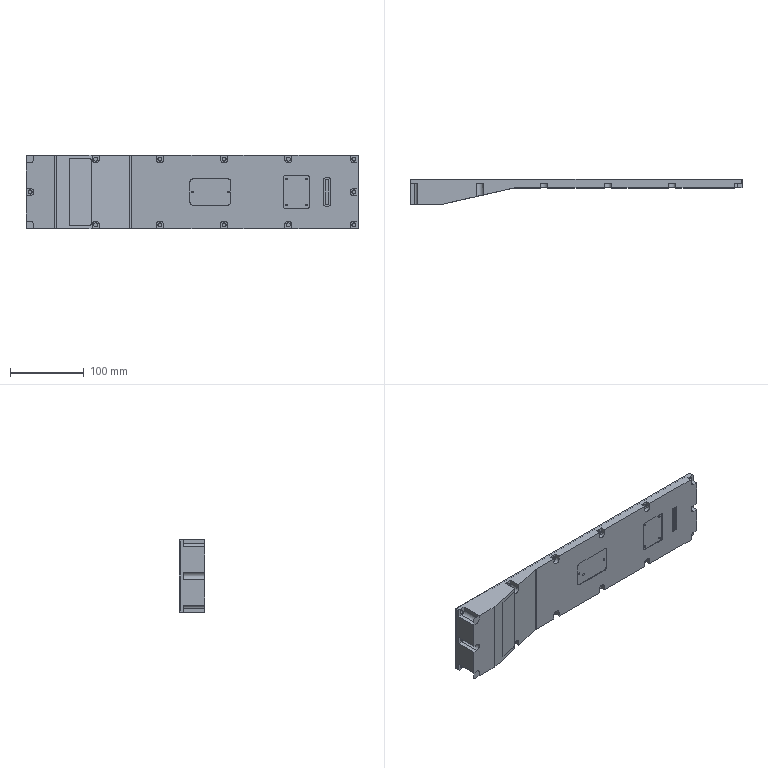Part | 1 solid | 372 faces | box 450 x 35 x 100 mm | volume 304861 mm3 | cylinder 180 | plane 128 | spline 36 | cone 28 | commonest cylinder face diameters 10 x64 2.5 x28 5.5 x28 4 x24 6 x24 8 x8